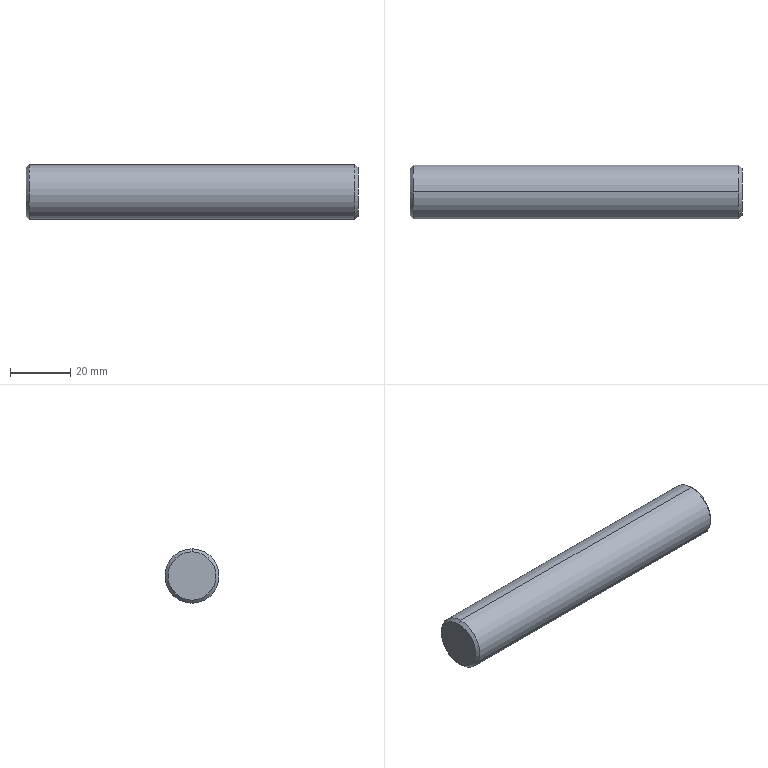Part | SolidWorks | features BaseBody 1 | 1 solid | 8 faces | box 110 x 18 x 18 mm | volume 27937 mm3 | cone 4 | cylinder 2 | plane 2 | commonest cylinder face diameters 18 x2
STEP:
#1=CARTESIAN_POINT('',(110.,0.,-8.));
#2=VERTEX_POINT('',#1);
#3=CARTESIAN_POINT('',(110.,0.,8.));
#4=VERTEX_POINT('',#3);
#5=CARTESIAN_POINT('',(110.,0.,0.));
#6=DIRECTION('',(1.,0.,0.));
#7=DIRECTION('',(0.,0.,-1.));
#8=AXIS2_PLACEMENT_3D('',#5,#6,#7);
#9=CIRCLE('',#8,8.);
#10=EDGE_CURVE('',#2,#4,#9,.T.);
#11=ORIENTED_EDGE('',*,*,#10,.F.);
#12=CARTESIAN_POINT('',(109.,0.,-9.));
#13=VERTEX_POINT('',#12);
#14=CARTESIAN_POINT('',(110.,0.,-8.));
#15=DIRECTION('',(-0.7071,0.,-0.7071));
#16=VECTOR('',#15,1000.);
#17=LINE('',#14,#16);
#18=EDGE_CURVE('',#2,#13,#17,.T.);
#19=ORIENTED_EDGE('',*,*,#18,.T.);
#20=CARTESIAN_POINT('',(109.,0.,9.));
#21=VERTEX_POINT('',#20);
#22=CARTESIAN_POINT('',(109.,0.,0.));
#23=DIRECTION('',(-1.,0.,0.));
#24=DIRECTION('',(0.,0.,-1.));
#25=AXIS2_PLACEMENT_3D('',#22,#23,#24);
#26=CIRCLE('',#25,9.);
#27=EDGE_CURVE('',#21,#13,#26,.T.);
#28=ORIENTED_EDGE('',*,*,#27,.F.);
#29=CARTESIAN_POINT('',(110.,0.,8.));
#30=DIRECTION('',(-0.7071,0.,0.7071));
#31=VECTOR('',#30,1000.);
#32=LINE('',#29,#31);
#33=EDGE_CURVE('',#4,#21,#32,.T.);
#34=ORIENTED_EDGE('',*,*,#33,.F.);
#35=EDGE_LOOP('',(#11,#19,#28,#34));
#36=FACE_OUTER_BOUND('',#35,.T.);
#37=CARTESIAN_POINT('',(110.,0.,0.));
#38=DIRECTION('',(-1.,0.,0.));
#39=DIRECTION('',(0.,0.,1.));
#40=AXIS2_PLACEMENT_3D('',#37,#38,#39);
#41=CONICAL_SURFACE('',#40,8.,0.7854);
#42=ADVANCED_FACE('',(#36),#41,.T.);
#43=CARTESIAN_POINT('',(0.,0.,8.));
#44=VERTEX_POINT('',#43);
#45=CARTESIAN_POINT('',(0.,0.,-8.));
#46=VERTEX_POINT('',#45);
#47=CARTESIAN_POINT('',(0.,0.,0.));
#48=DIRECTION('',(-1.,0.,0.));
#49=DIRECTION('',(0.,0.,-1.));
#50=AXIS2_PLACEMENT_3D('',#47,#48,#49);
#51=CIRCLE('',#50,8.);
#52=EDGE_CURVE('',#44,#46,#51,.T.);
#53=ORIENTED_EDGE('',*,*,#52,.F.);
#54=CARTESIAN_POINT('',(1.,0.,9.));
#55=VERTEX_POINT('',#54);
#56=CARTESIAN_POINT('',(1.,0.,9.));
#57=DIRECTION('',(0.7071,0.,0.7071));
#58=VECTOR('',#57,1000.);
#59=LINE('',#56,#58);
#60=EDGE_CURVE('',#44,#55,#59,.T.);
#61=ORIENTED_EDGE('',*,*,#60,.T.);
#62=CARTESIAN_POINT('',(1.,0.,-9.));
#63=VERTEX_POINT('',#62);
#64=CARTESIAN_POINT('',(1.,0.,0.));
#65=DIRECTION('',(1.,0.,0.));
#66=DIRECTION('',(0.,0.,-1.));
#67=AXIS2_PLACEMENT_3D('',#64,#65,#66);
#68=CIRCLE('',#67,9.);
#69=EDGE_CURVE('',#63,#55,#68,.T.);
#70=ORIENTED_EDGE('',*,*,#69,.F.);
#71=CARTESIAN_POINT('',(1.,0.,-9.));
#72=DIRECTION('',(0.7071,0.,-0.7071));
#73=VECTOR('',#72,1000.);
#74=LINE('',#71,#73);
#75=EDGE_CURVE('',#46,#63,#74,.T.);
#76=ORIENTED_EDGE('',*,*,#75,.F.);
#77=EDGE_LOOP('',(#53,#61,#70,#76));
#78=FACE_OUTER_BOUND('',#77,.T.);
#79=CARTESIAN_POINT('',(1.,0.,0.));
#80=DIRECTION('',(1.,0.,0.));
#81=DIRECTION('',(0.,0.,-1.));
#82=AXIS2_PLACEMENT_3D('',#79,#80,#81);
#83=CONICAL_SURFACE('',#82,9.,0.7854);
#84=ADVANCED_FACE('',(#78),#83,.T.);
#85=ORIENTED_EDGE('',*,*,#27,.T.);
#86=CARTESIAN_POINT('',(110.,0.,-9.));
#87=DIRECTION('',(-1.,0.,0.));
#88=VECTOR('',#87,1000.);
#89=LINE('',#86,#88);
#90=EDGE_CURVE('',#13,#63,#89,.T.);
#91=ORIENTED_EDGE('',*,*,#90,.T.);
#92=ORIENTED_EDGE('',*,*,#69,.T.);
#93=CARTESIAN_POINT('',(110.,0.,9.));
#94=DIRECTION('',(-1.,0.,0.));
#95=VECTOR('',#94,1000.);
#96=LINE('',#93,#95);
#97=EDGE_CURVE('',#21,#55,#96,.T.);
#98=ORIENTED_EDGE('',*,*,#97,.F.);
#99=EDGE_LOOP('',(#85,#91,#92,#98));
#100=FACE_OUTER_BOUND('',#99,.T.);
#101=CARTESIAN_POINT('',(110.,0.,0.));
#102=DIRECTION('',(-1.,0.,0.));
#103=DIRECTION('',(0.,0.,1.));
#104=AXIS2_PLACEMENT_3D('',#101,#102,#103);
#105=CYLINDRICAL_SURFACE('',#104,9.);
#106=ADVANCED_FACE('',(#100),#105,.T.);
#107=CARTESIAN_POINT('',(0.,0.,0.));
#108=DIRECTION('',(-1.,0.,0.));
#109=DIRECTION('',(0.,0.,-1.));
#110=AXIS2_PLACEMENT_3D('',#107,#108,#109);
#111=CIRCLE('',#110,8.);
#112=EDGE_CURVE('',#46,#44,#111,.T.);
#113=ORIENTED_EDGE('',*,*,#112,.T.);
#114=ORIENTED_EDGE('',*,*,#52,.T.);
#115=EDGE_LOOP('',(#113,#114));
#116=FACE_OUTER_BOUND('',#115,.T.);
#117=CARTESIAN_POINT('',(0.,0.,0.));
#118=DIRECTION('',(1.,0.,0.));
#119=DIRECTION('',(0.,1.,0.));
#120=AXIS2_PLACEMENT_3D('',#117,#118,#119);
#121=PLANE('',#120);
#122=ADVANCED_FACE('',(#116),#121,.F.);
#123=CARTESIAN_POINT('',(110.,0.,0.));
#124=DIRECTION('',(1.,0.,0.));
#125=DIRECTION('',(0.,0.,-1.));
#126=AXIS2_PLACEMENT_3D('',#123,#124,#125);
#127=CIRCLE('',#126,8.);
#128=EDGE_CURVE('',#4,#2,#127,.T.);
#129=ORIENTED_EDGE('',*,*,#128,.T.);
#130=ORIENTED_EDGE('',*,*,#10,.T.);
#131=EDGE_LOOP('',(#129,#130));
#132=FACE_OUTER_BOUND('',#131,.T.);
#133=CARTESIAN_POINT('',(110.,0.,0.));
#134=DIRECTION('',(1.,0.,0.));
#135=DIRECTION('',(0.,1.,0.));
#136=AXIS2_PLACEMENT_3D('',#133,#134,#135);
#137=PLANE('',#136);
#138=ADVANCED_FACE('',(#132),#137,.T.);
#139=ORIENTED_EDGE('',*,*,#90,.F.);
#140=CARTESIAN_POINT('',(109.,0.,0.));
#141=DIRECTION('',(-1.,0.,0.));
#142=DIRECTION('',(0.,0.,-1.));
#143=AXIS2_PLACEMENT_3D('',#140,#141,#142);
#144=CIRCLE('',#143,9.);
#145=EDGE_CURVE('',#13,#21,#144,.T.);
#146=ORIENTED_EDGE('',*,*,#145,.T.);
#147=ORIENTED_EDGE('',*,*,#97,.T.);
#148=CARTESIAN_POINT('',(1.,0.,0.));
#149=DIRECTION('',(1.,0.,0.));
#150=DIRECTION('',(0.,0.,-1.));
#151=AXIS2_PLACEMENT_3D('',#148,#149,#150);
#152=CIRCLE('',#151,9.);
#153=EDGE_CURVE('',#55,#63,#152,.T.);
#154=ORIENTED_EDGE('',*,*,#153,.T.);
#155=EDGE_LOOP('',(#139,#146,#147,#154));
#156=FACE_OUTER_BOUND('',#155,.T.);
#157=CARTESIAN_POINT('',(110.,0.,0.));
#158=DIRECTION('',(-1.,0.,0.));
#159=DIRECTION('',(0.,0.,1.));
#160=AXIS2_PLACEMENT_3D('',#157,#158,#159);
#161=CYLINDRICAL_SURFACE('',#160,9.);
#162=ADVANCED_FACE('',(#156),#161,.T.);
#163=ORIENTED_EDGE('',*,*,#60,.F.);
#164=ORIENTED_EDGE('',*,*,#112,.F.);
#165=ORIENTED_EDGE('',*,*,#75,.T.);
#166=ORIENTED_EDGE('',*,*,#153,.F.);
#167=EDGE_LOOP('',(#163,#164,#165,#166));
#168=FACE_OUTER_BOUND('',#167,.T.);
#169=CARTESIAN_POINT('',(1.,0.,0.));
#170=DIRECTION('',(1.,0.,0.));
#171=DIRECTION('',(0.,0.,-1.));
#172=AXIS2_PLACEMENT_3D('',#169,#170,#171);
#173=CONICAL_SURFACE('',#172,9.,0.7854);
#174=ADVANCED_FACE('',(#168),#173,.T.);
#175=ORIENTED_EDGE('',*,*,#18,.F.);
#176=ORIENTED_EDGE('',*,*,#128,.F.);
#177=ORIENTED_EDGE('',*,*,#33,.T.);
#178=ORIENTED_EDGE('',*,*,#145,.F.);
#179=EDGE_LOOP('',(#175,#176,#177,#178));
#180=FACE_OUTER_BOUND('',#179,.T.);
#181=CARTESIAN_POINT('',(110.,0.,0.));
#182=DIRECTION('',(-1.,0.,0.));
#183=DIRECTION('',(0.,0.,1.));
#184=AXIS2_PLACEMENT_3D('',#181,#182,#183);
#185=CONICAL_SURFACE('',#184,8.,0.7854);
#186=ADVANCED_FACE('',(#180),#185,.T.);
#187=CLOSED_SHELL('',(#42,#84,#106,#122,#138,#162,#174,#186));
#188=MANIFOLD_SOLID_BREP('',#187);
#189=CARTESIAN_POINT('',(0.,0.,0.));
#190=DIRECTION('',(0.,0.,1.));
#191=DIRECTION('',(1.,0.,0.));
#192=AXIS2_PLACEMENT_3D('',#189,#190,#191);
#193=(LENGTH_UNIT()NAMED_UNIT(*)SI_UNIT(.MILLI.,.METRE.));
#194=UNCERTAINTY_MEASURE_WITH_UNIT(LENGTH_MEASURE(0.00001),#193,'','');
#195=(NAMED_UNIT(*)PLANE_ANGLE_UNIT()SI_UNIT($,.RADIAN.));
#196=(NAMED_UNIT(*)SI_UNIT($,.STERADIAN.)SOLID_ANGLE_UNIT());
#197=(GEOMETRIC_REPRESENTATION_CONTEXT(3)GLOBAL_UNCERTAINTY_ASSIGNED_CONTEXT((#194))GLOBAL_UNIT_ASSIGNED_CONTEXT((#193,#195,#196))REPRESENTATION_CONTEXT('',''));
#198=ADVANCED_BREP_SHAPE_REPRESENTATION('',(#188,#192),#197);